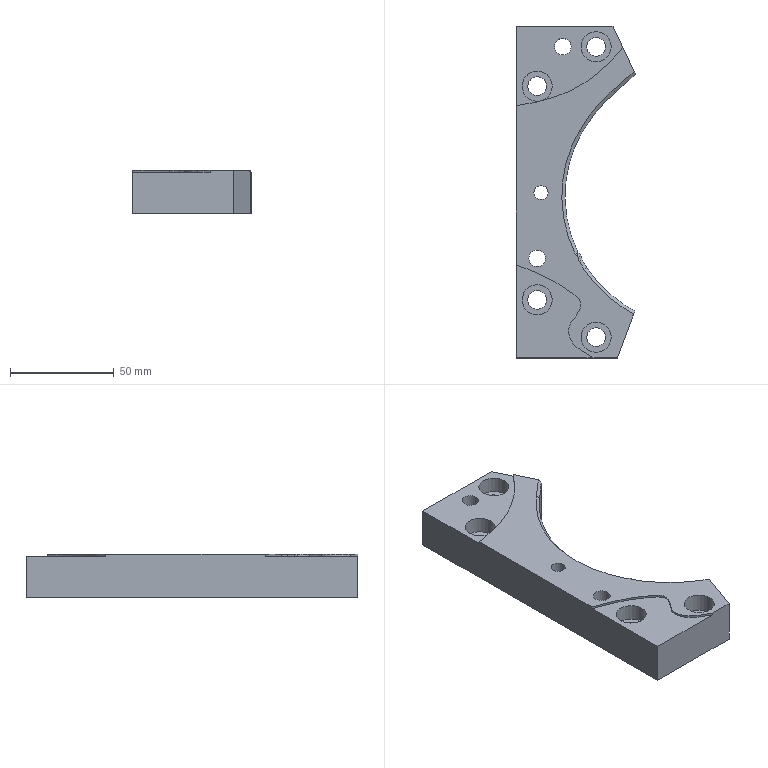Part | NX | features 23 2 | 1 solid | 55 faces | box 57.406 x 160 x 21 mm | volume 117065 mm3 | plane 21 | cylinder 15 | spline 14 | cone 5 | commonest cylinder face diameters 9 x4 14.5 x4 8.001 x2 6.8 x1 127.148 x1 140.96 x1